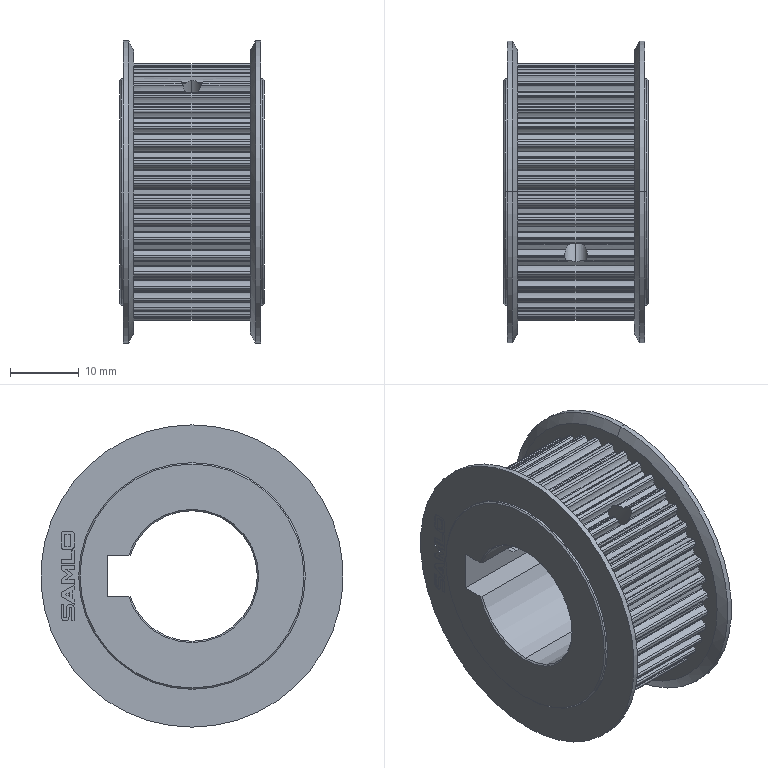Part | SolidWorks | features BaseBody 1 | 1 solid | 478 faces | box 21 x 44 x 44 mm | volume 16333 mm3 | cylinder 403 | plane 61 | cone 14 | commonest cylinder face diameters 0.56 x103 0.3 x97 3.95 x90 35.22 x43 37.44 x41 0.442 x4